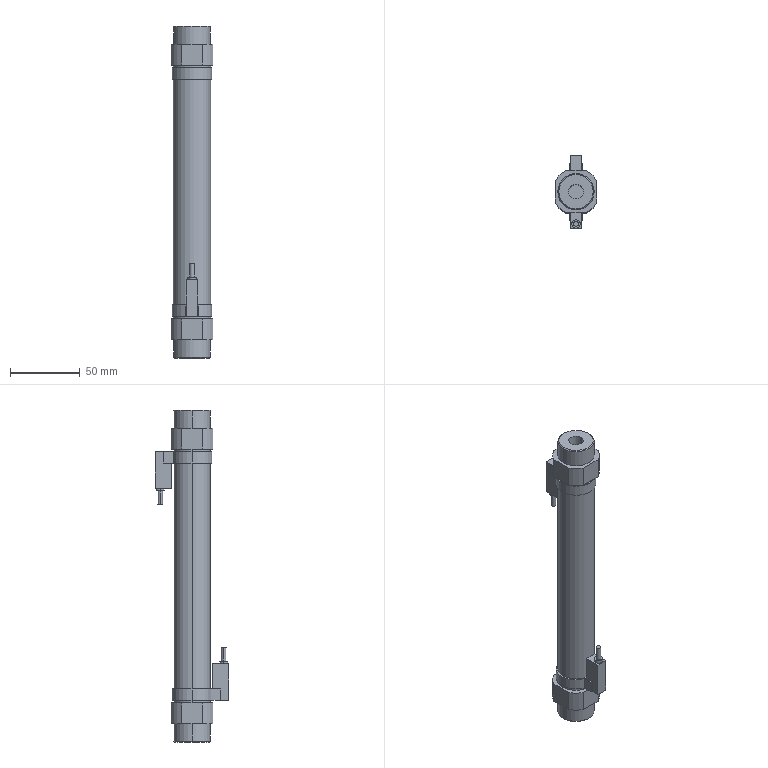Part | STEP file | A_CDM2B25-150-C76(0)_Default | 1 solid | 97 faces | box 30 x 52.6 x 238 mm | volume 131860 mm3 | plane 45 | cylinder 40 | cone 8 | spline 4 | commonest cylinder face diameters 28.6 x8 33.5 x8 26.6 x6 3.4 x4 6 x4 8.57 x4